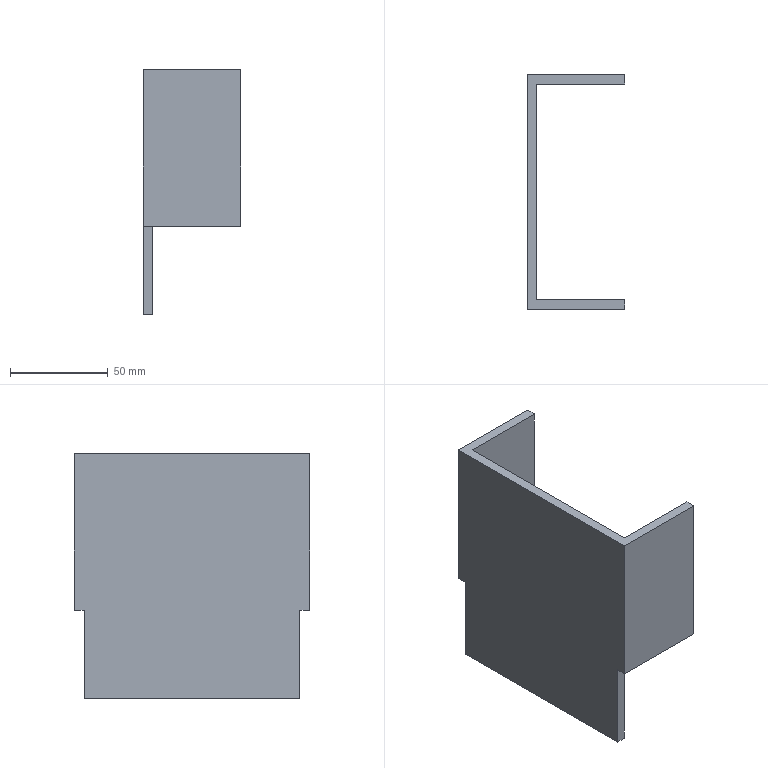Part | SolidWorks | features Cut 3, Extrusion 1, ICE 1 | 1 solid | 14 faces | box 50 x 120 x 125 mm | volume 108750 mm3 | plane 14
STEP:
#1=CARTESIAN_POINT('',(0.,0.,-80.));
#2=VERTEX_POINT('',#1);
#3=CARTESIAN_POINT('',(0.,0.,0.));
#4=VERTEX_POINT('',#3);
#5=CARTESIAN_POINT('',(0.,0.,-150.));
#6=DIRECTION('',(0.,0.,1.));
#7=VECTOR('',#6,1000.);
#8=LINE('',#5,#7);
#9=EDGE_CURVE('',#2,#4,#8,.T.);
#10=ORIENTED_EDGE('',*,*,#9,.F.);
#11=CARTESIAN_POINT('',(50.,0.,-80.));
#12=VERTEX_POINT('',#11);
#13=CARTESIAN_POINT('',(50.,0.,-80.));
#14=DIRECTION('',(-1.,0.,0.));
#15=VECTOR('',#14,1000.);
#16=LINE('',#13,#15);
#17=EDGE_CURVE('',#12,#2,#16,.T.);
#18=ORIENTED_EDGE('',*,*,#17,.F.);
#19=CARTESIAN_POINT('',(50.,0.,0.));
#20=VERTEX_POINT('',#19);
#21=CARTESIAN_POINT('',(50.,0.,-150.));
#22=DIRECTION('',(0.,0.,1.));
#23=VECTOR('',#22,1000.);
#24=LINE('',#21,#23);
#25=EDGE_CURVE('',#12,#20,#24,.T.);
#26=ORIENTED_EDGE('',*,*,#25,.T.);
#27=CARTESIAN_POINT('',(0.,0.,0.));
#28=DIRECTION('',(1.,0.,0.));
#29=VECTOR('',#28,1000.);
#30=LINE('',#27,#29);
#31=EDGE_CURVE('',#4,#20,#30,.T.);
#32=ORIENTED_EDGE('',*,*,#31,.F.);
#33=EDGE_LOOP('',(#10,#18,#26,#32));
#34=FACE_OUTER_BOUND('',#33,.T.);
#35=CARTESIAN_POINT('',(0.,0.,-150.));
#36=DIRECTION('',(0.,-1.,0.));
#37=DIRECTION('',(0.,0.,-1.));
#38=AXIS2_PLACEMENT_3D('',#35,#36,#37);
#39=PLANE('',#38);
#40=ADVANCED_FACE('',(#34),#39,.T.);
#41=CARTESIAN_POINT('',(50.,5.,-80.));
#42=VERTEX_POINT('',#41);
#43=CARTESIAN_POINT('',(50.,5.,0.));
#44=VERTEX_POINT('',#43);
#45=CARTESIAN_POINT('',(50.,5.,-150.));
#46=DIRECTION('',(0.,0.,1.));
#47=VECTOR('',#46,1000.);
#48=LINE('',#45,#47);
#49=EDGE_CURVE('',#42,#44,#48,.T.);
#50=ORIENTED_EDGE('',*,*,#49,.F.);
#51=CARTESIAN_POINT('',(5.,5.,-80.));
#52=VERTEX_POINT('',#51);
#53=CARTESIAN_POINT('',(5.,5.,-80.));
#54=DIRECTION('',(1.,0.,0.));
#55=VECTOR('',#54,1000.);
#56=LINE('',#53,#55);
#57=EDGE_CURVE('',#52,#42,#56,.T.);
#58=ORIENTED_EDGE('',*,*,#57,.F.);
#59=CARTESIAN_POINT('',(5.,5.,0.));
#60=VERTEX_POINT('',#59);
#61=CARTESIAN_POINT('',(5.,5.,-150.));
#62=DIRECTION('',(0.,0.,1.));
#63=VECTOR('',#62,1000.);
#64=LINE('',#61,#63);
#65=EDGE_CURVE('',#52,#60,#64,.T.);
#66=ORIENTED_EDGE('',*,*,#65,.T.);
#67=CARTESIAN_POINT('',(5.,5.,0.));
#68=DIRECTION('',(-1.,0.,0.));
#69=VECTOR('',#68,1000.);
#70=LINE('',#67,#69);
#71=EDGE_CURVE('',#44,#60,#70,.T.);
#72=ORIENTED_EDGE('',*,*,#71,.F.);
#73=EDGE_LOOP('',(#50,#58,#66,#72));
#74=FACE_OUTER_BOUND('',#73,.T.);
#75=CARTESIAN_POINT('',(5.,5.,-150.));
#76=DIRECTION('',(0.,1.,0.));
#77=DIRECTION('',(0.,0.,1.));
#78=AXIS2_PLACEMENT_3D('',#75,#76,#77);
#79=PLANE('',#78);
#80=ADVANCED_FACE('',(#74),#79,.T.);
#81=ORIENTED_EDGE('',*,*,#25,.F.);
#82=CARTESIAN_POINT('',(50.,5.,-80.));
#83=DIRECTION('',(0.,-1.,0.));
#84=VECTOR('',#83,1000.);
#85=LINE('',#82,#84);
#86=EDGE_CURVE('',#42,#12,#85,.T.);
#87=ORIENTED_EDGE('',*,*,#86,.F.);
#88=ORIENTED_EDGE('',*,*,#49,.T.);
#89=CARTESIAN_POINT('',(50.,0.,0.));
#90=DIRECTION('',(0.,1.,0.));
#91=VECTOR('',#90,1000.);
#92=LINE('',#89,#91);
#93=EDGE_CURVE('',#20,#44,#92,.T.);
#94=ORIENTED_EDGE('',*,*,#93,.F.);
#95=EDGE_LOOP('',(#81,#87,#88,#94));
#96=FACE_OUTER_BOUND('',#95,.T.);
#97=CARTESIAN_POINT('',(50.,0.,-150.));
#98=DIRECTION('',(1.,0.,0.));
#99=DIRECTION('',(0.,0.,-1.));
#100=AXIS2_PLACEMENT_3D('',#97,#98,#99);
#101=PLANE('',#100);
#102=ADVANCED_FACE('',(#96),#101,.T.);
#103=CARTESIAN_POINT('',(50.,120.,-80.));
#104=VERTEX_POINT('',#103);
#105=CARTESIAN_POINT('',(50.,120.,0.));
#106=VERTEX_POINT('',#105);
#107=CARTESIAN_POINT('',(50.,120.,-150.));
#108=DIRECTION('',(0.,0.,1.));
#109=VECTOR('',#108,1000.);
#110=LINE('',#107,#109);
#111=EDGE_CURVE('',#104,#106,#110,.T.);
#112=ORIENTED_EDGE('',*,*,#111,.F.);
#113=CARTESIAN_POINT('',(0.,120.,-80.));
#114=VERTEX_POINT('',#113);
#115=CARTESIAN_POINT('',(0.,120.,-80.));
#116=DIRECTION('',(1.,0.,0.));
#117=VECTOR('',#116,1000.);
#118=LINE('',#115,#117);
#119=EDGE_CURVE('',#114,#104,#118,.T.);
#120=ORIENTED_EDGE('',*,*,#119,.F.);
#121=CARTESIAN_POINT('',(0.,120.,0.));
#122=VERTEX_POINT('',#121);
#123=CARTESIAN_POINT('',(0.,120.,-150.));
#124=DIRECTION('',(0.,0.,1.));
#125=VECTOR('',#124,1000.);
#126=LINE('',#123,#125);
#127=EDGE_CURVE('',#114,#122,#126,.T.);
#128=ORIENTED_EDGE('',*,*,#127,.T.);
#129=CARTESIAN_POINT('',(0.,120.,0.));
#130=DIRECTION('',(-1.,0.,0.));
#131=VECTOR('',#130,1000.);
#132=LINE('',#129,#131);
#133=EDGE_CURVE('',#106,#122,#132,.T.);
#134=ORIENTED_EDGE('',*,*,#133,.F.);
#135=EDGE_LOOP('',(#112,#120,#128,#134));
#136=FACE_OUTER_BOUND('',#135,.T.);
#137=CARTESIAN_POINT('',(0.,120.,-150.));
#138=DIRECTION('',(0.,1.,0.));
#139=DIRECTION('',(0.,0.,1.));
#140=AXIS2_PLACEMENT_3D('',#137,#138,#139);
#141=PLANE('',#140);
#142=ADVANCED_FACE('',(#136),#141,.T.);
#143=CARTESIAN_POINT('',(50.,115.,-80.));
#144=VERTEX_POINT('',#143);
#145=CARTESIAN_POINT('',(50.,115.,0.));
#146=VERTEX_POINT('',#145);
#147=CARTESIAN_POINT('',(50.,115.,-150.));
#148=DIRECTION('',(0.,0.,1.));
#149=VECTOR('',#148,1000.);
#150=LINE('',#147,#149);
#151=EDGE_CURVE('',#144,#146,#150,.T.);
#152=ORIENTED_EDGE('',*,*,#151,.F.);
#153=CARTESIAN_POINT('',(50.,120.,-80.));
#154=DIRECTION('',(0.,-1.,0.));
#155=VECTOR('',#154,1000.);
#156=LINE('',#153,#155);
#157=EDGE_CURVE('',#104,#144,#156,.T.);
#158=ORIENTED_EDGE('',*,*,#157,.F.);
#159=ORIENTED_EDGE('',*,*,#111,.T.);
#160=CARTESIAN_POINT('',(50.,115.,0.));
#161=DIRECTION('',(0.,1.,0.));
#162=VECTOR('',#161,1000.);
#163=LINE('',#160,#162);
#164=EDGE_CURVE('',#146,#106,#163,.T.);
#165=ORIENTED_EDGE('',*,*,#164,.F.);
#166=EDGE_LOOP('',(#152,#158,#159,#165));
#167=FACE_OUTER_BOUND('',#166,.T.);
#168=CARTESIAN_POINT('',(50.,115.,-150.));
#169=DIRECTION('',(1.,0.,0.));
#170=DIRECTION('',(0.,0.,-1.));
#171=AXIS2_PLACEMENT_3D('',#168,#169,#170);
#172=PLANE('',#171);
#173=ADVANCED_FACE('',(#167),#172,.T.);
#174=CARTESIAN_POINT('',(5.,115.,-80.));
#175=VERTEX_POINT('',#174);
#176=CARTESIAN_POINT('',(5.,115.,0.));
#177=VERTEX_POINT('',#176);
#178=CARTESIAN_POINT('',(5.,115.,-150.));
#179=DIRECTION('',(0.,0.,1.));
#180=VECTOR('',#179,1000.);
#181=LINE('',#178,#180);
#182=EDGE_CURVE('',#175,#177,#181,.T.);
#183=ORIENTED_EDGE('',*,*,#182,.F.);
#184=CARTESIAN_POINT('',(50.,115.,-80.));
#185=DIRECTION('',(-1.,0.,0.));
#186=VECTOR('',#185,1000.);
#187=LINE('',#184,#186);
#188=EDGE_CURVE('',#144,#175,#187,.T.);
#189=ORIENTED_EDGE('',*,*,#188,.F.);
#190=ORIENTED_EDGE('',*,*,#151,.T.);
#191=CARTESIAN_POINT('',(5.,115.,0.));
#192=DIRECTION('',(1.,0.,0.));
#193=VECTOR('',#192,1000.);
#194=LINE('',#191,#193);
#195=EDGE_CURVE('',#177,#146,#194,.T.);
#196=ORIENTED_EDGE('',*,*,#195,.F.);
#197=EDGE_LOOP('',(#183,#189,#190,#196));
#198=FACE_OUTER_BOUND('',#197,.T.);
#199=CARTESIAN_POINT('',(5.,115.,-150.));
#200=DIRECTION('',(0.,-1.,0.));
#201=DIRECTION('',(0.,0.,-1.));
#202=AXIS2_PLACEMENT_3D('',#199,#200,#201);
#203=PLANE('',#202);
#204=ADVANCED_FACE('',(#198),#203,.T.);
#205=CARTESIAN_POINT('',(0.,5.,-80.));
#206=VERTEX_POINT('',#205);
#207=CARTESIAN_POINT('',(0.,5.,-125.));
#208=VERTEX_POINT('',#207);
#209=CARTESIAN_POINT('',(0.,5.,-105.));
#210=DIRECTION('',(0.,0.,-1.));
#211=VECTOR('',#210,1000.);
#212=LINE('',#209,#211);
#213=EDGE_CURVE('',#206,#208,#212,.T.);
#214=ORIENTED_EDGE('',*,*,#213,.F.);
#215=CARTESIAN_POINT('',(0.,0.,-80.));
#216=DIRECTION('',(0.,1.,0.));
#217=VECTOR('',#216,1000.);
#218=LINE('',#215,#217);
#219=EDGE_CURVE('',#2,#206,#218,.T.);
#220=ORIENTED_EDGE('',*,*,#219,.F.);
#221=ORIENTED_EDGE('',*,*,#9,.T.);
#222=CARTESIAN_POINT('',(0.,0.,0.));
#223=DIRECTION('',(0.,-1.,0.));
#224=VECTOR('',#223,1000.);
#225=LINE('',#222,#224);
#226=EDGE_CURVE('',#122,#4,#225,.T.);
#227=ORIENTED_EDGE('',*,*,#226,.F.);
#228=ORIENTED_EDGE('',*,*,#127,.F.);
#229=CARTESIAN_POINT('',(0.,115.,-80.));
#230=VERTEX_POINT('',#229);
#231=CARTESIAN_POINT('',(0.,115.,-80.));
#232=DIRECTION('',(0.,1.,0.));
#233=VECTOR('',#232,1000.);
#234=LINE('',#231,#233);
#235=EDGE_CURVE('',#230,#114,#234,.T.);
#236=ORIENTED_EDGE('',*,*,#235,.F.);
#237=CARTESIAN_POINT('',(0.,115.,-125.));
#238=VERTEX_POINT('',#237);
#239=CARTESIAN_POINT('',(0.,115.,-105.));
#240=DIRECTION('',(0.,0.,-1.));
#241=VECTOR('',#240,1000.);
#242=LINE('',#239,#241);
#243=EDGE_CURVE('',#230,#238,#242,.T.);
#244=ORIENTED_EDGE('',*,*,#243,.T.);
#245=CARTESIAN_POINT('',(0.,5.,-125.));
#246=DIRECTION('',(0.,1.,0.));
#247=VECTOR('',#246,1000.);
#248=LINE('',#245,#247);
#249=EDGE_CURVE('',#208,#238,#248,.T.);
#250=ORIENTED_EDGE('',*,*,#249,.F.);
#251=EDGE_LOOP('',(#214,#220,#221,#227,#228,#236,#244,#250));
#252=FACE_OUTER_BOUND('',#251,.T.);
#253=CARTESIAN_POINT('',(0.,0.,-150.));
#254=DIRECTION('',(-1.,0.,0.));
#255=DIRECTION('',(0.,0.,1.));
#256=AXIS2_PLACEMENT_3D('',#253,#254,#255);
#257=PLANE('',#256);
#258=ADVANCED_FACE('',(#252),#257,.T.);
#259=CARTESIAN_POINT('',(5.,5.,-125.));
#260=VERTEX_POINT('',#259);
#261=CARTESIAN_POINT('',(5.,5.,-150.));
#262=DIRECTION('',(0.,0.,1.));
#263=VECTOR('',#262,1000.);
#264=LINE('',#261,#263);
#265=EDGE_CURVE('',#260,#52,#264,.T.);
#266=ORIENTED_EDGE('',*,*,#265,.F.);
#267=CARTESIAN_POINT('',(5.,115.,-125.));
#268=VERTEX_POINT('',#267);
#269=CARTESIAN_POINT('',(5.,115.,-125.));
#270=DIRECTION('',(0.,-1.,0.));
#271=VECTOR('',#270,1000.);
#272=LINE('',#269,#271);
#273=EDGE_CURVE('',#268,#260,#272,.T.);
#274=ORIENTED_EDGE('',*,*,#273,.F.);
#275=CARTESIAN_POINT('',(5.,115.,-150.));
#276=DIRECTION('',(0.,0.,1.));
#277=VECTOR('',#276,1000.);
#278=LINE('',#275,#277);
#279=EDGE_CURVE('',#268,#175,#278,.T.);
#280=ORIENTED_EDGE('',*,*,#279,.T.);
#281=ORIENTED_EDGE('',*,*,#182,.T.);
#282=CARTESIAN_POINT('',(5.,5.,0.));
#283=DIRECTION('',(0.,1.,0.));
#284=VECTOR('',#283,1000.);
#285=LINE('',#282,#284);
#286=EDGE_CURVE('',#60,#177,#285,.T.);
#287=ORIENTED_EDGE('',*,*,#286,.F.);
#288=ORIENTED_EDGE('',*,*,#65,.F.);
#289=EDGE_LOOP('',(#266,#274,#280,#281,#287,#288));
#290=FACE_OUTER_BOUND('',#289,.T.);
#291=CARTESIAN_POINT('',(5.,5.,-150.));
#292=DIRECTION('',(1.,0.,0.));
#293=DIRECTION('',(0.,0.,-1.));
#294=AXIS2_PLACEMENT_3D('',#291,#292,#293);
#295=PLANE('',#294);
#296=ADVANCED_FACE('',(#290),#295,.T.);
#297=CARTESIAN_POINT('',(0.,115.,-125.));
#298=DIRECTION('',(1.,0.,0.));
#299=VECTOR('',#298,1000.);
#300=LINE('',#297,#299);
#301=EDGE_CURVE('',#238,#268,#300,.T.);
#302=ORIENTED_EDGE('',*,*,#301,.F.);
#303=ORIENTED_EDGE('',*,*,#243,.F.);
#304=CARTESIAN_POINT('',(50.,115.,-80.));
#305=DIRECTION('',(-1.,0.,0.));
#306=VECTOR('',#305,1000.);
#307=LINE('',#304,#306);
#308=EDGE_CURVE('',#175,#230,#307,.T.);
#309=ORIENTED_EDGE('',*,*,#308,.F.);
#310=ORIENTED_EDGE('',*,*,#279,.F.);
#311=EDGE_LOOP('',(#302,#303,#309,#310));
#312=FACE_OUTER_BOUND('',#311,.T.);
#313=CARTESIAN_POINT('',(0.,115.,-105.));
#314=DIRECTION('',(0.,-1.,0.));
#315=DIRECTION('',(0.,0.,-1.));
#316=AXIS2_PLACEMENT_3D('',#313,#314,#315);
#317=PLANE('',#316);
#318=ADVANCED_FACE('',(#312),#317,.F.);
#319=CARTESIAN_POINT('',(5.,5.,-125.));
#320=DIRECTION('',(-1.,0.,0.));
#321=VECTOR('',#320,1000.);
#322=LINE('',#319,#321);
#323=EDGE_CURVE('',#260,#208,#322,.T.);
#324=ORIENTED_EDGE('',*,*,#323,.F.);
#325=ORIENTED_EDGE('',*,*,#265,.T.);
#326=CARTESIAN_POINT('',(5.,5.,-80.));
#327=DIRECTION('',(1.,0.,0.));
#328=VECTOR('',#327,1000.);
#329=LINE('',#326,#328);
#330=EDGE_CURVE('',#206,#52,#329,.T.);
#331=ORIENTED_EDGE('',*,*,#330,.F.);
#332=ORIENTED_EDGE('',*,*,#213,.T.);
#333=EDGE_LOOP('',(#324,#325,#331,#332));
#334=FACE_OUTER_BOUND('',#333,.T.);
#335=CARTESIAN_POINT('',(50.,5.,-105.));
#336=DIRECTION('',(0.,1.,0.));
#337=DIRECTION('',(-1.,0.,0.));
#338=AXIS2_PLACEMENT_3D('',#335,#336,#337);
#339=PLANE('',#338);
#340=ADVANCED_FACE('',(#334),#339,.F.);
#341=ORIENTED_EDGE('',*,*,#31,.T.);
#342=ORIENTED_EDGE('',*,*,#93,.T.);
#343=ORIENTED_EDGE('',*,*,#71,.T.);
#344=ORIENTED_EDGE('',*,*,#286,.T.);
#345=ORIENTED_EDGE('',*,*,#195,.T.);
#346=ORIENTED_EDGE('',*,*,#164,.T.);
#347=ORIENTED_EDGE('',*,*,#133,.T.);
#348=ORIENTED_EDGE('',*,*,#226,.T.);
#349=EDGE_LOOP('',(#341,#342,#343,#344,#345,#346,#347,#348));
#350=FACE_OUTER_BOUND('',#349,.T.);
#351=CARTESIAN_POINT('',(0.,0.,0.));
#352=DIRECTION('',(0.,0.,1.));
#353=DIRECTION('',(1.,0.,0.));
#354=AXIS2_PLACEMENT_3D('',#351,#352,#353);
#355=PLANE('',#354);
#356=ADVANCED_FACE('',(#350),#355,.T.);
#357=ORIENTED_EDGE('',*,*,#301,.T.);
#358=ORIENTED_EDGE('',*,*,#273,.T.);
#359=ORIENTED_EDGE('',*,*,#323,.T.);
#360=ORIENTED_EDGE('',*,*,#249,.T.);
#361=EDGE_LOOP('',(#357,#358,#359,#360));
#362=FACE_OUTER_BOUND('',#361,.T.);
#363=CARTESIAN_POINT('',(0.,0.,-125.));
#364=DIRECTION('',(0.,0.,-1.));
#365=DIRECTION('',(-1.,0.,0.));
#366=AXIS2_PLACEMENT_3D('',#363,#364,#365);
#367=PLANE('',#366);
#368=ADVANCED_FACE('',(#362),#367,.T.);
#369=ORIENTED_EDGE('',*,*,#119,.T.);
#370=ORIENTED_EDGE('',*,*,#157,.T.);
#371=ORIENTED_EDGE('',*,*,#188,.T.);
#372=ORIENTED_EDGE('',*,*,#308,.T.);
#373=ORIENTED_EDGE('',*,*,#235,.T.);
#374=EDGE_LOOP('',(#369,#370,#371,#372,#373));
#375=FACE_OUTER_BOUND('',#374,.T.);
#376=CARTESIAN_POINT('',(0.,0.,-80.));
#377=DIRECTION('',(0.,0.,-1.));
#378=DIRECTION('',(-1.,0.,0.));
#379=AXIS2_PLACEMENT_3D('',#376,#377,#378);
#380=PLANE('',#379);
#381=ADVANCED_FACE('',(#375),#380,.T.);
#382=ORIENTED_EDGE('',*,*,#330,.T.);
#383=ORIENTED_EDGE('',*,*,#57,.T.);
#384=ORIENTED_EDGE('',*,*,#86,.T.);
#385=ORIENTED_EDGE('',*,*,#17,.T.);
#386=ORIENTED_EDGE('',*,*,#219,.T.);
#387=EDGE_LOOP('',(#382,#383,#384,#385,#386));
#388=FACE_OUTER_BOUND('',#387,.T.);
#389=CARTESIAN_POINT('',(0.,0.,-80.));
#390=DIRECTION('',(0.,0.,-1.));
#391=DIRECTION('',(-1.,0.,0.));
#392=AXIS2_PLACEMENT_3D('',#389,#390,#391);
#393=PLANE('',#392);
#394=ADVANCED_FACE('',(#388),#393,.T.);
#395=CLOSED_SHELL('',(#40,#80,#102,#142,#173,#204,#258,#296,#318,#340,#356,#368,#381,#394));
#396=MANIFOLD_SOLID_BREP('',#395);
#397=CARTESIAN_POINT('',(0.,0.,0.));
#398=DIRECTION('',(0.,0.,1.));
#399=DIRECTION('',(1.,0.,0.));
#400=AXIS2_PLACEMENT_3D('',#397,#398,#399);
#401=(LENGTH_UNIT()NAMED_UNIT(*)SI_UNIT(.MILLI.,.METRE.));
#402=UNCERTAINTY_MEASURE_WITH_UNIT(LENGTH_MEASURE(0.00001),#401,'','');
#403=(NAMED_UNIT(*)PLANE_ANGLE_UNIT()SI_UNIT($,.RADIAN.));
#404=(NAMED_UNIT(*)SI_UNIT($,.STERADIAN.)SOLID_ANGLE_UNIT());
#405=(GEOMETRIC_REPRESENTATION_CONTEXT(3)GLOBAL_UNCERTAINTY_ASSIGNED_CONTEXT((#402))GLOBAL_UNIT_ASSIGNED_CONTEXT((#401,#403,#404))REPRESENTATION_CONTEXT('',''));
#406=ADVANCED_BREP_SHAPE_REPRESENTATION('',(#396,#400),#405);